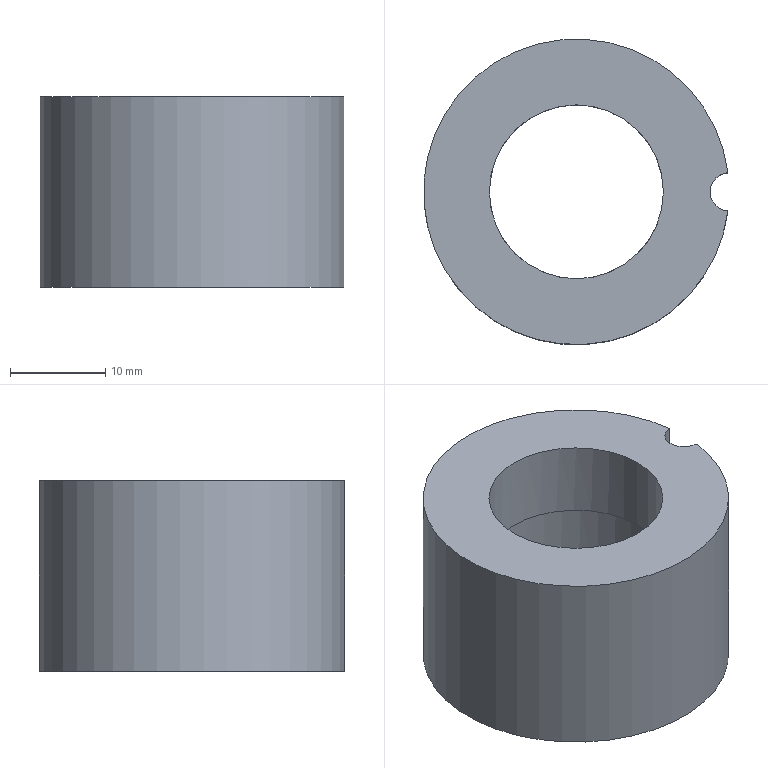Part | NX | features solid 2 | 1 solid | 7 faces | box 31.875 x 32 x 20 mm | volume 9877 mm3 | cylinder 4 | plane 3 | commonest cylinder face diameters 4 x1 18.22 x1 20.6 x1 32 x1
STEP:
#1=CARTESIAN_POINT('',(420.876,8.346,-5.264));
#2=VERTEX_POINT('',#1);
#3=CARTESIAN_POINT('',(420.876,12.338,-5.264));
#4=VERTEX_POINT('',#3);
#5=CARTESIAN_POINT('',(421.001,10.342,-5.264));
#6=DIRECTION('',(0.,0.,-1.));
#7=DIRECTION('',(-1.,0.,0.));
#8=AXIS2_PLACEMENT_3D('',#5,#6,#7);
#9=CIRCLE('',#8,2.);
#10=EDGE_CURVE('',#2,#4,#9,.T.);
#11=ORIENTED_EDGE('',*,*,#10,.T.);
#12=CARTESIAN_POINT('',(405.001,10.342,-5.264));
#13=DIRECTION('',(0.,0.,-1.));
#14=DIRECTION('',(-1.,0.,0.));
#15=AXIS2_PLACEMENT_3D('',#12,#13,#14);
#16=CIRCLE('',#15,16.);
#17=EDGE_CURVE('',#2,#4,#16,.T.);
#18=ORIENTED_EDGE('',*,*,#17,.F.);
#19=EDGE_LOOP('',(#11,#18));
#20=FACE_BOUND('',#19,.T.);
#21=CARTESIAN_POINT('',(395.891,10.342,-5.264));
#22=VERTEX_POINT('',#21);
#23=CARTESIAN_POINT('',(405.001,10.342,-5.264));
#24=DIRECTION('',(0.,0.,-1.));
#25=DIRECTION('',(-1.,0.,0.));
#26=AXIS2_PLACEMENT_3D('',#23,#24,#25);
#27=CIRCLE('',#26,9.11);
#28=EDGE_CURVE('',#22,#22,#27,.T.);
#29=ORIENTED_EDGE('',*,*,#28,.T.);
#30=EDGE_LOOP('',(#29));
#31=FACE_BOUND('',#30,.T.);
#32=CARTESIAN_POINT('',(405.001,10.342,-5.264));
#33=DIRECTION('',(0.,0.,1.));
#34=DIRECTION('',(1.,0.,0.));
#35=AXIS2_PLACEMENT_3D('',#32,#33,#34);
#36=PLANE('',#35);
#37=ADVANCED_FACE('',(#20,#31),#36,.T.);
#38=CARTESIAN_POINT('',(420.876,12.338,-25.264));
#39=VERTEX_POINT('',#38);
#40=CARTESIAN_POINT('',(420.876,8.346,-25.264));
#41=VERTEX_POINT('',#40);
#42=CARTESIAN_POINT('',(421.001,10.342,-25.264));
#43=DIRECTION('',(0.,0.,1.));
#44=DIRECTION('',(1.,0.,0.));
#45=AXIS2_PLACEMENT_3D('',#42,#43,#44);
#46=CIRCLE('',#45,2.);
#47=EDGE_CURVE('',#39,#41,#46,.T.);
#48=ORIENTED_EDGE('',*,*,#47,.T.);
#49=CARTESIAN_POINT('',(405.001,10.342,-25.264));
#50=DIRECTION('',(0.,0.,1.));
#51=DIRECTION('',(1.,0.,0.));
#52=AXIS2_PLACEMENT_3D('',#49,#50,#51);
#53=CIRCLE('',#52,16.);
#54=EDGE_CURVE('',#39,#41,#53,.T.);
#55=ORIENTED_EDGE('',*,*,#54,.F.);
#56=EDGE_LOOP('',(#48,#55));
#57=FACE_BOUND('',#56,.T.);
#58=CARTESIAN_POINT('',(415.301,10.342,-25.264));
#59=VERTEX_POINT('',#58);
#60=CARTESIAN_POINT('',(405.001,10.342,-25.264));
#61=DIRECTION('',(0.,0.,1.));
#62=DIRECTION('',(1.,0.,0.));
#63=AXIS2_PLACEMENT_3D('',#60,#61,#62);
#64=CIRCLE('',#63,10.3);
#65=EDGE_CURVE('',#59,#59,#64,.T.);
#66=ORIENTED_EDGE('',*,*,#65,.T.);
#67=EDGE_LOOP('',(#66));
#68=FACE_BOUND('',#67,.T.);
#69=CARTESIAN_POINT('',(405.001,10.342,-25.264));
#70=DIRECTION('',(0.,0.,-1.));
#71=DIRECTION('',(-1.,0.,0.));
#72=AXIS2_PLACEMENT_3D('',#69,#70,#71);
#73=PLANE('',#72);
#74=ADVANCED_FACE('',(#57,#68),#73,.T.);
#75=CARTESIAN_POINT('',(420.876,12.338,-15.264));
#76=DIRECTION('',(0.,0.,1.));
#77=VECTOR('',#76,1000.);
#78=LINE('',#75,#77);
#79=EDGE_CURVE('',#39,#4,#78,.T.);
#80=ORIENTED_EDGE('',*,*,#79,.F.);
#81=ORIENTED_EDGE('',*,*,#54,.T.);
#82=CARTESIAN_POINT('',(420.876,8.346,-15.264));
#83=DIRECTION('',(0.,0.,1.));
#84=VECTOR('',#83,1000.);
#85=LINE('',#82,#84);
#86=EDGE_CURVE('',#2,#41,#85,.F.);
#87=ORIENTED_EDGE('',*,*,#86,.F.);
#88=ORIENTED_EDGE('',*,*,#17,.T.);
#89=EDGE_LOOP('',(#80,#81,#87,#88));
#90=FACE_BOUND('',#89,.T.);
#91=CARTESIAN_POINT('',(405.001,10.342,-25.264));
#92=DIRECTION('',(0.,0.,1.));
#93=DIRECTION('',(1.,0.,0.));
#94=AXIS2_PLACEMENT_3D('',#91,#92,#93);
#95=CYLINDRICAL_SURFACE('',#94,16.);
#96=ADVANCED_FACE('',(#90),#95,.T.);
#97=CARTESIAN_POINT('',(414.111,10.342,-13.264));
#98=VERTEX_POINT('',#97);
#99=CARTESIAN_POINT('',(405.001,10.342,-13.264));
#100=DIRECTION('',(0.,0.,1.));
#101=DIRECTION('',(1.,0.,0.));
#102=AXIS2_PLACEMENT_3D('',#99,#100,#101);
#103=CIRCLE('',#102,9.11);
#104=EDGE_CURVE('',#98,#98,#103,.T.);
#105=ORIENTED_EDGE('',*,*,#104,.T.);
#106=EDGE_LOOP('',(#105));
#107=FACE_BOUND('',#106,.T.);
#108=CARTESIAN_POINT('',(394.701,10.342,-13.264));
#109=VERTEX_POINT('',#108);
#110=CARTESIAN_POINT('',(405.001,10.342,-13.264));
#111=DIRECTION('',(0.,0.,-1.));
#112=DIRECTION('',(-1.,0.,0.));
#113=AXIS2_PLACEMENT_3D('',#110,#111,#112);
#114=CIRCLE('',#113,10.3);
#115=EDGE_CURVE('',#109,#109,#114,.T.);
#116=ORIENTED_EDGE('',*,*,#115,.T.);
#117=EDGE_LOOP('',(#116));
#118=FACE_BOUND('',#117,.T.);
#119=CARTESIAN_POINT('',(405.001,10.342,-13.264));
#120=DIRECTION('',(0.,0.,1.));
#121=DIRECTION('',(1.,0.,0.));
#122=AXIS2_PLACEMENT_3D('',#119,#120,#121);
#123=PLANE('',#122);
#124=ADVANCED_FACE('',(#107,#118),#123,.F.);
#125=ORIENTED_EDGE('',*,*,#115,.F.);
#126=EDGE_LOOP('',(#125));
#127=FACE_BOUND('',#126,.T.);
#128=ORIENTED_EDGE('',*,*,#65,.F.);
#129=EDGE_LOOP('',(#128));
#130=FACE_BOUND('',#129,.T.);
#131=CARTESIAN_POINT('',(405.001,10.342,-25.264));
#132=DIRECTION('',(0.,0.,1.));
#133=DIRECTION('',(1.,0.,0.));
#134=AXIS2_PLACEMENT_3D('',#131,#132,#133);
#135=CYLINDRICAL_SURFACE('',#134,10.3);
#136=ADVANCED_FACE('',(#127,#130),#135,.F.);
#137=ORIENTED_EDGE('',*,*,#28,.F.);
#138=EDGE_LOOP('',(#137));
#139=FACE_BOUND('',#138,.T.);
#140=ORIENTED_EDGE('',*,*,#104,.F.);
#141=EDGE_LOOP('',(#140));
#142=FACE_BOUND('',#141,.T.);
#143=CARTESIAN_POINT('',(405.001,10.342,-13.264));
#144=DIRECTION('',(0.,0.,1.));
#145=DIRECTION('',(1.,0.,0.));
#146=AXIS2_PLACEMENT_3D('',#143,#144,#145);
#147=CYLINDRICAL_SURFACE('',#146,9.11);
#148=ADVANCED_FACE('',(#139,#142),#147,.F.);
#149=ORIENTED_EDGE('',*,*,#79,.T.);
#150=ORIENTED_EDGE('',*,*,#10,.F.);
#151=ORIENTED_EDGE('',*,*,#86,.T.);
#152=ORIENTED_EDGE('',*,*,#47,.F.);
#153=EDGE_LOOP('',(#149,#150,#151,#152));
#154=FACE_BOUND('',#153,.T.);
#155=CARTESIAN_POINT('',(421.001,10.342,-25.264));
#156=DIRECTION('',(0.,0.,1.));
#157=DIRECTION('',(1.,0.,0.));
#158=AXIS2_PLACEMENT_3D('',#155,#156,#157);
#159=CYLINDRICAL_SURFACE('',#158,2.);
#160=ADVANCED_FACE('',(#154),#159,.F.);
#161=CLOSED_SHELL('',(#37,#74,#96,#124,#136,#148,#160));
#162=MANIFOLD_SOLID_BREP('',#161);
#163=(LENGTH_UNIT()NAMED_UNIT(*)SI_UNIT(.MILLI.,.METRE.));
#164=UNCERTAINTY_MEASURE_WITH_UNIT(LENGTH_MEASURE(0.00001),#163,'','');
#165=(NAMED_UNIT(*)PLANE_ANGLE_UNIT()SI_UNIT($,.RADIAN.));
#166=(NAMED_UNIT(*)SI_UNIT($,.STERADIAN.)SOLID_ANGLE_UNIT());
#167=(GEOMETRIC_REPRESENTATION_CONTEXT(3)GLOBAL_UNCERTAINTY_ASSIGNED_CONTEXT((#164))GLOBAL_UNIT_ASSIGNED_CONTEXT((#163,#165,#166))REPRESENTATION_CONTEXT('',''));
#168=ADVANCED_BREP_SHAPE_REPRESENTATION('',(#162),#167);